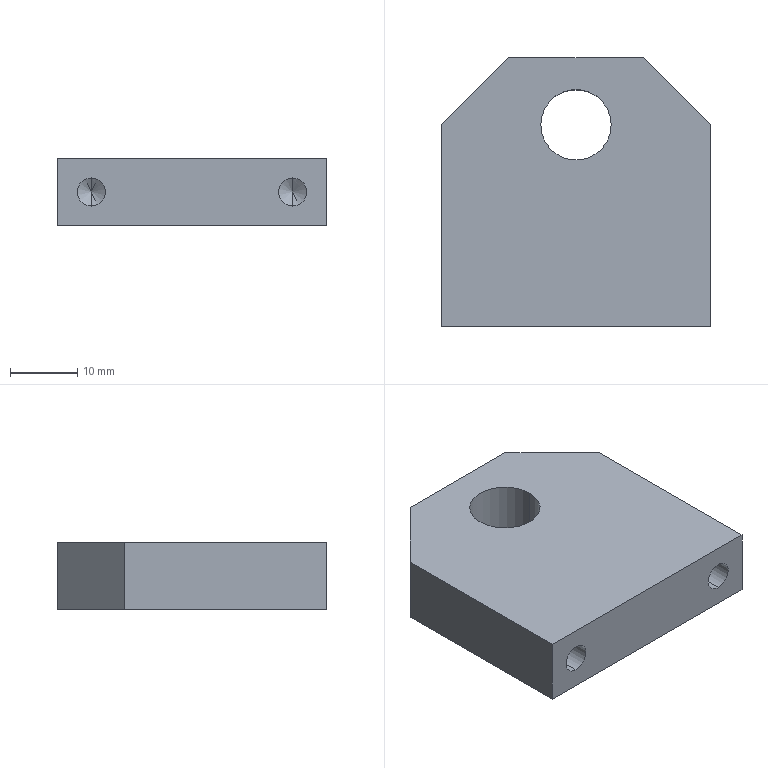Part | SolidWorks | features BaseBody 1 | 1 solid | 18 faces | box 40 x 40 x 10 mm | volume 13735 mm3 | plane 8 | cylinder 6 | cone 4 | commonest cylinder face diameters 4.2 x4 10.5 x2
STEP:
#1=CARTESIAN_POINT('',(-15.,-6.,7.1));
#2=VERTEX_POINT('',#1);
#3=CARTESIAN_POINT('',(-15.,-6.,2.9));
#4=VERTEX_POINT('',#3);
#5=CARTESIAN_POINT('',(-15.,-6.,5.));
#6=DIRECTION('',(0.,-1.,0.));
#7=DIRECTION('',(0.,0.,-1.));
#8=AXIS2_PLACEMENT_3D('',#5,#6,#7);
#9=CIRCLE('',#8,2.1);
#10=EDGE_CURVE('',#2,#4,#9,.T.);
#11=ORIENTED_EDGE('',*,*,#10,.F.);
#12=CARTESIAN_POINT('',(-15.,-20.,7.1));
#13=VERTEX_POINT('',#12);
#14=CARTESIAN_POINT('',(-15.,-20.,7.1));
#15=DIRECTION('',(0.,-1.,0.));
#16=VECTOR('',#15,1000.);
#17=LINE('',#14,#16);
#18=EDGE_CURVE('',#2,#13,#17,.T.);
#19=ORIENTED_EDGE('',*,*,#18,.T.);
#20=CARTESIAN_POINT('',(-15.,-20.,2.9));
#21=VERTEX_POINT('',#20);
#22=CARTESIAN_POINT('',(-15.,-20.,5.));
#23=DIRECTION('',(0.,-1.,0.));
#24=DIRECTION('',(0.,0.,-1.));
#25=AXIS2_PLACEMENT_3D('',#22,#23,#24);
#26=CIRCLE('',#25,2.1);
#27=EDGE_CURVE('',#13,#21,#26,.T.);
#28=ORIENTED_EDGE('',*,*,#27,.T.);
#29=CARTESIAN_POINT('',(-15.,-20.,2.9));
#30=DIRECTION('',(0.,-1.,0.));
#31=VECTOR('',#30,1000.);
#32=LINE('',#29,#31);
#33=EDGE_CURVE('',#4,#21,#32,.T.);
#34=ORIENTED_EDGE('',*,*,#33,.F.);
#35=EDGE_LOOP('',(#11,#19,#28,#34));
#36=FACE_OUTER_BOUND('',#35,.T.);
#37=CARTESIAN_POINT('',(-15.,-20.,5.));
#38=DIRECTION('',(0.,-1.,0.));
#39=DIRECTION('',(0.,0.,-1.));
#40=AXIS2_PLACEMENT_3D('',#37,#38,#39);
#41=CYLINDRICAL_SURFACE('',#40,2.1);
#42=ADVANCED_FACE('',(#36),#41,.F.);
#43=CARTESIAN_POINT('',(-15.,-4.738,5.));
#44=VERTEX_POINT('',#43);
#45=CARTESIAN_POINT('',(-15.,-6.,2.9));
#46=DIRECTION('',(0.,-0.515,-0.8572));
#47=VECTOR('',#46,1000.);
#48=LINE('',#45,#47);
#49=EDGE_CURVE('',#44,#4,#48,.T.);
#50=ORIENTED_EDGE('',*,*,#49,.F.);
#51=CARTESIAN_POINT('',(-15.,-6.,7.1));
#52=DIRECTION('',(0.,-0.515,0.8572));
#53=VECTOR('',#52,1000.);
#54=LINE('',#51,#53);
#55=EDGE_CURVE('',#44,#2,#54,.T.);
#56=ORIENTED_EDGE('',*,*,#55,.T.);
#57=ORIENTED_EDGE('',*,*,#10,.T.);
#58=EDGE_LOOP('',(#50,#56,#57));
#59=FACE_OUTER_BOUND('',#58,.T.);
#60=CARTESIAN_POINT('',(-15.,-6.,5.));
#61=DIRECTION('',(0.,-1.,0.));
#62=DIRECTION('',(0.,0.,-1.));
#63=AXIS2_PLACEMENT_3D('',#60,#61,#62);
#64=CONICAL_SURFACE('',#63,2.1,1.03);
#65=ADVANCED_FACE('',(#59),#64,.F.);
#66=CARTESIAN_POINT('',(15.,-6.,7.1));
#67=VERTEX_POINT('',#66);
#68=CARTESIAN_POINT('',(15.,-6.,2.9));
#69=VERTEX_POINT('',#68);
#70=CARTESIAN_POINT('',(15.,-6.,5.));
#71=DIRECTION('',(0.,-1.,0.));
#72=DIRECTION('',(0.,0.,-1.));
#73=AXIS2_PLACEMENT_3D('',#70,#71,#72);
#74=CIRCLE('',#73,2.1);
#75=EDGE_CURVE('',#67,#69,#74,.T.);
#76=ORIENTED_EDGE('',*,*,#75,.F.);
#77=CARTESIAN_POINT('',(15.,-20.,7.1));
#78=VERTEX_POINT('',#77);
#79=CARTESIAN_POINT('',(15.,-20.,7.1));
#80=DIRECTION('',(0.,-1.,0.));
#81=VECTOR('',#80,1000.);
#82=LINE('',#79,#81);
#83=EDGE_CURVE('',#67,#78,#82,.T.);
#84=ORIENTED_EDGE('',*,*,#83,.T.);
#85=CARTESIAN_POINT('',(15.,-20.,2.9));
#86=VERTEX_POINT('',#85);
#87=CARTESIAN_POINT('',(15.,-20.,5.));
#88=DIRECTION('',(0.,-1.,0.));
#89=DIRECTION('',(0.,0.,-1.));
#90=AXIS2_PLACEMENT_3D('',#87,#88,#89);
#91=CIRCLE('',#90,2.1);
#92=EDGE_CURVE('',#78,#86,#91,.T.);
#93=ORIENTED_EDGE('',*,*,#92,.T.);
#94=CARTESIAN_POINT('',(15.,-20.,2.9));
#95=DIRECTION('',(0.,-1.,0.));
#96=VECTOR('',#95,1000.);
#97=LINE('',#94,#96);
#98=EDGE_CURVE('',#69,#86,#97,.T.);
#99=ORIENTED_EDGE('',*,*,#98,.F.);
#100=EDGE_LOOP('',(#76,#84,#93,#99));
#101=FACE_OUTER_BOUND('',#100,.T.);
#102=CARTESIAN_POINT('',(15.,-20.,5.));
#103=DIRECTION('',(0.,-1.,0.));
#104=DIRECTION('',(0.,0.,-1.));
#105=AXIS2_PLACEMENT_3D('',#102,#103,#104);
#106=CYLINDRICAL_SURFACE('',#105,2.1);
#107=ADVANCED_FACE('',(#101),#106,.F.);
#108=CARTESIAN_POINT('',(15.,-4.738,5.));
#109=VERTEX_POINT('',#108);
#110=CARTESIAN_POINT('',(15.,-6.,2.9));
#111=DIRECTION('',(0.,-0.515,-0.8572));
#112=VECTOR('',#111,1000.);
#113=LINE('',#110,#112);
#114=EDGE_CURVE('',#109,#69,#113,.T.);
#115=ORIENTED_EDGE('',*,*,#114,.F.);
#116=CARTESIAN_POINT('',(15.,-6.,7.1));
#117=DIRECTION('',(0.,-0.515,0.8572));
#118=VECTOR('',#117,1000.);
#119=LINE('',#116,#118);
#120=EDGE_CURVE('',#109,#67,#119,.T.);
#121=ORIENTED_EDGE('',*,*,#120,.T.);
#122=ORIENTED_EDGE('',*,*,#75,.T.);
#123=EDGE_LOOP('',(#115,#121,#122));
#124=FACE_OUTER_BOUND('',#123,.T.);
#125=CARTESIAN_POINT('',(15.,-6.,5.));
#126=DIRECTION('',(0.,-1.,0.));
#127=DIRECTION('',(0.,0.,-1.));
#128=AXIS2_PLACEMENT_3D('',#125,#126,#127);
#129=CONICAL_SURFACE('',#128,2.1,1.03);
#130=ADVANCED_FACE('',(#124),#129,.F.);
#131=CARTESIAN_POINT('',(-5.25,10.,0.));
#132=VERTEX_POINT('',#131);
#133=CARTESIAN_POINT('',(5.25,10.,0.));
#134=VERTEX_POINT('',#133);
#135=CARTESIAN_POINT('',(0.,10.,0.));
#136=DIRECTION('',(0.,0.,1.));
#137=DIRECTION('',(1.,0.,0.));
#138=AXIS2_PLACEMENT_3D('',#135,#136,#137);
#139=CIRCLE('',#138,5.25);
#140=EDGE_CURVE('',#132,#134,#139,.T.);
#141=ORIENTED_EDGE('',*,*,#140,.F.);
#142=CARTESIAN_POINT('',(-5.25,10.,10.));
#143=VERTEX_POINT('',#142);
#144=CARTESIAN_POINT('',(-5.25,10.,0.));
#145=DIRECTION('',(0.,0.,1.));
#146=VECTOR('',#145,1000.);
#147=LINE('',#144,#146);
#148=EDGE_CURVE('',#132,#143,#147,.T.);
#149=ORIENTED_EDGE('',*,*,#148,.T.);
#150=CARTESIAN_POINT('',(5.25,10.,10.));
#151=VERTEX_POINT('',#150);
#152=CARTESIAN_POINT('',(0.,10.,10.));
#153=DIRECTION('',(0.,0.,1.));
#154=DIRECTION('',(1.,0.,0.));
#155=AXIS2_PLACEMENT_3D('',#152,#153,#154);
#156=CIRCLE('',#155,5.25);
#157=EDGE_CURVE('',#143,#151,#156,.T.);
#158=ORIENTED_EDGE('',*,*,#157,.T.);
#159=CARTESIAN_POINT('',(5.25,10.,0.));
#160=DIRECTION('',(0.,0.,1.));
#161=VECTOR('',#160,1000.);
#162=LINE('',#159,#161);
#163=EDGE_CURVE('',#134,#151,#162,.T.);
#164=ORIENTED_EDGE('',*,*,#163,.F.);
#165=EDGE_LOOP('',(#141,#149,#158,#164));
#166=FACE_OUTER_BOUND('',#165,.T.);
#167=CARTESIAN_POINT('',(0.,10.,0.));
#168=DIRECTION('',(0.,0.,1.));
#169=DIRECTION('',(1.,0.,0.));
#170=AXIS2_PLACEMENT_3D('',#167,#168,#169);
#171=CYLINDRICAL_SURFACE('',#170,5.25);
#172=ADVANCED_FACE('',(#166),#171,.F.);
#173=CARTESIAN_POINT('',(-20.,10.,10.));
#174=VERTEX_POINT('',#173);
#175=CARTESIAN_POINT('',(-20.,-20.,10.));
#176=VERTEX_POINT('',#175);
#177=CARTESIAN_POINT('',(-20.,-20.,10.));
#178=DIRECTION('',(0.,-1.,0.));
#179=VECTOR('',#178,1000.);
#180=LINE('',#177,#179);
#181=EDGE_CURVE('',#174,#176,#180,.T.);
#182=ORIENTED_EDGE('',*,*,#181,.F.);
#183=CARTESIAN_POINT('',(-20.,10.,0.));
#184=VERTEX_POINT('',#183);
#185=CARTESIAN_POINT('',(-20.,10.,10.));
#186=DIRECTION('',(0.,0.,-1.));
#187=VECTOR('',#186,1000.);
#188=LINE('',#185,#187);
#189=EDGE_CURVE('',#174,#184,#188,.T.);
#190=ORIENTED_EDGE('',*,*,#189,.T.);
#191=CARTESIAN_POINT('',(-20.,-20.,0.));
#192=VERTEX_POINT('',#191);
#193=CARTESIAN_POINT('',(-20.,-20.,0.));
#194=DIRECTION('',(0.,-1.,0.));
#195=VECTOR('',#194,1000.);
#196=LINE('',#193,#195);
#197=EDGE_CURVE('',#184,#192,#196,.T.);
#198=ORIENTED_EDGE('',*,*,#197,.T.);
#199=CARTESIAN_POINT('',(-20.,-20.,10.));
#200=DIRECTION('',(0.,0.,-1.));
#201=VECTOR('',#200,1000.);
#202=LINE('',#199,#201);
#203=EDGE_CURVE('',#176,#192,#202,.T.);
#204=ORIENTED_EDGE('',*,*,#203,.F.);
#205=EDGE_LOOP('',(#182,#190,#198,#204));
#206=FACE_OUTER_BOUND('',#205,.T.);
#207=CARTESIAN_POINT('',(-20.,-20.,10.));
#208=DIRECTION('',(1.,0.,0.));
#209=DIRECTION('',(0.,0.,-1.));
#210=AXIS2_PLACEMENT_3D('',#207,#208,#209);
#211=PLANE('',#210);
#212=ADVANCED_FACE('',(#206),#211,.F.);
#213=CARTESIAN_POINT('',(-15.,-20.,5.));
#214=DIRECTION('',(0.,-1.,0.));
#215=DIRECTION('',(0.,0.,-1.));
#216=AXIS2_PLACEMENT_3D('',#213,#214,#215);
#217=CIRCLE('',#216,2.1);
#218=EDGE_CURVE('',#21,#13,#217,.T.);
#219=ORIENTED_EDGE('',*,*,#218,.F.);
#220=ORIENTED_EDGE('',*,*,#27,.F.);
#221=EDGE_LOOP('',(#219,#220));
#222=FACE_BOUND('',#221,.T.);
#223=CARTESIAN_POINT('',(15.,-20.,5.));
#224=DIRECTION('',(0.,-1.,0.));
#225=DIRECTION('',(0.,0.,-1.));
#226=AXIS2_PLACEMENT_3D('',#223,#224,#225);
#227=CIRCLE('',#226,2.1);
#228=EDGE_CURVE('',#86,#78,#227,.T.);
#229=ORIENTED_EDGE('',*,*,#228,.F.);
#230=ORIENTED_EDGE('',*,*,#92,.F.);
#231=EDGE_LOOP('',(#229,#230));
#232=FACE_BOUND('',#231,.T.);
#233=CARTESIAN_POINT('',(20.,-20.,0.));
#234=VERTEX_POINT('',#233);
#235=CARTESIAN_POINT('',(20.,-20.,0.));
#236=DIRECTION('',(1.,0.,0.));
#237=VECTOR('',#236,1000.);
#238=LINE('',#235,#237);
#239=EDGE_CURVE('',#192,#234,#238,.T.);
#240=ORIENTED_EDGE('',*,*,#239,.T.);
#241=CARTESIAN_POINT('',(20.,-20.,10.));
#242=VERTEX_POINT('',#241);
#243=CARTESIAN_POINT('',(20.,-20.,10.));
#244=DIRECTION('',(0.,0.,-1.));
#245=VECTOR('',#244,1000.);
#246=LINE('',#243,#245);
#247=EDGE_CURVE('',#242,#234,#246,.T.);
#248=ORIENTED_EDGE('',*,*,#247,.F.);
#249=CARTESIAN_POINT('',(20.,-20.,10.));
#250=DIRECTION('',(1.,0.,0.));
#251=VECTOR('',#250,1000.);
#252=LINE('',#249,#251);
#253=EDGE_CURVE('',#176,#242,#252,.T.);
#254=ORIENTED_EDGE('',*,*,#253,.F.);
#255=ORIENTED_EDGE('',*,*,#203,.T.);
#256=EDGE_LOOP('',(#240,#248,#254,#255));
#257=FACE_OUTER_BOUND('',#256,.T.);
#258=CARTESIAN_POINT('',(20.,-20.,10.));
#259=DIRECTION('',(0.,1.,0.));
#260=DIRECTION('',(-1.,0.,0.));
#261=AXIS2_PLACEMENT_3D('',#258,#259,#260);
#262=PLANE('',#261);
#263=ADVANCED_FACE('',(#222,#232,#257),#262,.F.);
#264=CARTESIAN_POINT('',(20.,10.,0.));
#265=VERTEX_POINT('',#264);
#266=CARTESIAN_POINT('',(20.,-20.,0.));
#267=DIRECTION('',(0.,1.,0.));
#268=VECTOR('',#267,1000.);
#269=LINE('',#266,#268);
#270=EDGE_CURVE('',#234,#265,#269,.T.);
#271=ORIENTED_EDGE('',*,*,#270,.T.);
#272=CARTESIAN_POINT('',(20.,10.,10.));
#273=VERTEX_POINT('',#272);
#274=CARTESIAN_POINT('',(20.,10.,10.));
#275=DIRECTION('',(0.,0.,1.));
#276=VECTOR('',#275,1000.);
#277=LINE('',#274,#276);
#278=EDGE_CURVE('',#265,#273,#277,.T.);
#279=ORIENTED_EDGE('',*,*,#278,.T.);
#280=CARTESIAN_POINT('',(20.,-20.,10.));
#281=DIRECTION('',(0.,1.,0.));
#282=VECTOR('',#281,1000.);
#283=LINE('',#280,#282);
#284=EDGE_CURVE('',#242,#273,#283,.T.);
#285=ORIENTED_EDGE('',*,*,#284,.F.);
#286=ORIENTED_EDGE('',*,*,#247,.T.);
#287=EDGE_LOOP('',(#271,#279,#285,#286));
#288=FACE_OUTER_BOUND('',#287,.T.);
#289=CARTESIAN_POINT('',(20.,-20.,10.));
#290=DIRECTION('',(-1.,0.,0.));
#291=DIRECTION('',(0.,0.,1.));
#292=AXIS2_PLACEMENT_3D('',#289,#290,#291);
#293=PLANE('',#292);
#294=ADVANCED_FACE('',(#288),#293,.F.);
#295=CARTESIAN_POINT('',(10.,20.,10.));
#296=VERTEX_POINT('',#295);
#297=CARTESIAN_POINT('',(-10.,20.,10.));
#298=VERTEX_POINT('',#297);
#299=CARTESIAN_POINT('',(20.,20.,10.));
#300=DIRECTION('',(-1.,0.,0.));
#301=VECTOR('',#300,1000.);
#302=LINE('',#299,#301);
#303=EDGE_CURVE('',#296,#298,#302,.T.);
#304=ORIENTED_EDGE('',*,*,#303,.F.);
#305=CARTESIAN_POINT('',(10.,20.,0.));
#306=VERTEX_POINT('',#305);
#307=CARTESIAN_POINT('',(10.,20.,10.));
#308=DIRECTION('',(0.,0.,-1.));
#309=VECTOR('',#308,1000.);
#310=LINE('',#307,#309);
#311=EDGE_CURVE('',#296,#306,#310,.T.);
#312=ORIENTED_EDGE('',*,*,#311,.T.);
#313=CARTESIAN_POINT('',(-10.,20.,0.));
#314=VERTEX_POINT('',#313);
#315=CARTESIAN_POINT('',(20.,20.,0.));
#316=DIRECTION('',(-1.,0.,0.));
#317=VECTOR('',#316,1000.);
#318=LINE('',#315,#317);
#319=EDGE_CURVE('',#306,#314,#318,.T.);
#320=ORIENTED_EDGE('',*,*,#319,.T.);
#321=CARTESIAN_POINT('',(-10.,20.,10.));
#322=DIRECTION('',(0.,0.,1.));
#323=VECTOR('',#322,1000.);
#324=LINE('',#321,#323);
#325=EDGE_CURVE('',#314,#298,#324,.T.);
#326=ORIENTED_EDGE('',*,*,#325,.T.);
#327=EDGE_LOOP('',(#304,#312,#320,#326));
#328=FACE_OUTER_BOUND('',#327,.T.);
#329=CARTESIAN_POINT('',(20.,20.,10.));
#330=DIRECTION('',(0.,-1.,0.));
#331=DIRECTION('',(1.,0.,0.));
#332=AXIS2_PLACEMENT_3D('',#329,#330,#331);
#333=PLANE('',#332);
#334=ADVANCED_FACE('',(#328),#333,.F.);
#335=CARTESIAN_POINT('',(0.,10.,10.));
#336=DIRECTION('',(0.,0.,1.));
#337=DIRECTION('',(1.,0.,0.));
#338=AXIS2_PLACEMENT_3D('',#335,#336,#337);
#339=CIRCLE('',#338,5.25);
#340=EDGE_CURVE('',#151,#143,#339,.T.);
#341=ORIENTED_EDGE('',*,*,#340,.F.);
#342=ORIENTED_EDGE('',*,*,#157,.F.);
#343=EDGE_LOOP('',(#341,#342));
#344=FACE_BOUND('',#343,.T.);
#345=ORIENTED_EDGE('',*,*,#284,.T.);
#346=CARTESIAN_POINT('',(15.,15.,10.));
#347=DIRECTION('',(-0.7071,0.7071,0.));
#348=VECTOR('',#347,1000.);
#349=LINE('',#346,#348);
#350=EDGE_CURVE('',#273,#296,#349,.T.);
#351=ORIENTED_EDGE('',*,*,#350,.T.);
#352=ORIENTED_EDGE('',*,*,#303,.T.);
#353=CARTESIAN_POINT('',(-15.,15.,10.));
#354=DIRECTION('',(-0.7071,-0.7071,0.));
#355=VECTOR('',#354,1000.);
#356=LINE('',#353,#355);
#357=EDGE_CURVE('',#298,#174,#356,.T.);
#358=ORIENTED_EDGE('',*,*,#357,.T.);
#359=ORIENTED_EDGE('',*,*,#181,.T.);
#360=ORIENTED_EDGE('',*,*,#253,.T.);
#361=EDGE_LOOP('',(#345,#351,#352,#358,#359,#360));
#362=FACE_OUTER_BOUND('',#361,.T.);
#363=CARTESIAN_POINT('',(0.,0.,10.));
#364=DIRECTION('',(0.,0.,1.));
#365=DIRECTION('',(1.,0.,0.));
#366=AXIS2_PLACEMENT_3D('',#363,#364,#365);
#367=PLANE('',#366);
#368=ADVANCED_FACE('',(#344,#362),#367,.T.);
#369=CARTESIAN_POINT('',(0.,10.,0.));
#370=DIRECTION('',(0.,0.,1.));
#371=DIRECTION('',(1.,0.,0.));
#372=AXIS2_PLACEMENT_3D('',#369,#370,#371);
#373=CIRCLE('',#372,5.25);
#374=EDGE_CURVE('',#134,#132,#373,.T.);
#375=ORIENTED_EDGE('',*,*,#374,.T.);
#376=ORIENTED_EDGE('',*,*,#140,.T.);
#377=EDGE_LOOP('',(#375,#376));
#378=FACE_BOUND('',#377,.T.);
#379=ORIENTED_EDGE('',*,*,#319,.F.);
#380=CARTESIAN_POINT('',(10.,20.,0.));
#381=DIRECTION('',(0.7071,-0.7071,0.));
#382=VECTOR('',#381,1000.);
#383=LINE('',#380,#382);
#384=EDGE_CURVE('',#306,#265,#383,.T.);
#385=ORIENTED_EDGE('',*,*,#384,.T.);
#386=ORIENTED_EDGE('',*,*,#270,.F.);
#387=ORIENTED_EDGE('',*,*,#239,.F.);
#388=ORIENTED_EDGE('',*,*,#197,.F.);
#389=CARTESIAN_POINT('',(-20.,10.,0.));
#390=DIRECTION('',(0.7071,0.7071,0.));
#391=VECTOR('',#390,1000.);
#392=LINE('',#389,#391);
#393=EDGE_CURVE('',#184,#314,#392,.T.);
#394=ORIENTED_EDGE('',*,*,#393,.T.);
#395=EDGE_LOOP('',(#379,#385,#386,#387,#388,#394));
#396=FACE_OUTER_BOUND('',#395,.T.);
#397=CARTESIAN_POINT('',(0.,0.,0.));
#398=DIRECTION('',(0.,0.,1.));
#399=DIRECTION('',(1.,0.,0.));
#400=AXIS2_PLACEMENT_3D('',#397,#398,#399);
#401=PLANE('',#400);
#402=ADVANCED_FACE('',(#378,#396),#401,.F.);
#403=ORIENTED_EDGE('',*,*,#148,.F.);
#404=ORIENTED_EDGE('',*,*,#374,.F.);
#405=ORIENTED_EDGE('',*,*,#163,.T.);
#406=ORIENTED_EDGE('',*,*,#340,.T.);
#407=EDGE_LOOP('',(#403,#404,#405,#406));
#408=FACE_OUTER_BOUND('',#407,.T.);
#409=CARTESIAN_POINT('',(0.,10.,0.));
#410=DIRECTION('',(0.,0.,1.));
#411=DIRECTION('',(1.,0.,0.));
#412=AXIS2_PLACEMENT_3D('',#409,#410,#411);
#413=CYLINDRICAL_SURFACE('',#412,5.25);
#414=ADVANCED_FACE('',(#408),#413,.F.);
#415=ORIENTED_EDGE('',*,*,#350,.F.);
#416=ORIENTED_EDGE('',*,*,#278,.F.);
#417=ORIENTED_EDGE('',*,*,#384,.F.);
#418=ORIENTED_EDGE('',*,*,#311,.F.);
#419=EDGE_LOOP('',(#415,#416,#417,#418));
#420=FACE_OUTER_BOUND('',#419,.T.);
#421=CARTESIAN_POINT('',(10.,20.,10.));
#422=DIRECTION('',(-0.7071,-0.7071,0.));
#423=DIRECTION('',(0.,0.,-1.));
#424=AXIS2_PLACEMENT_3D('',#421,#422,#423);
#425=PLANE('',#424);
#426=ADVANCED_FACE('',(#420),#425,.F.);
#427=ORIENTED_EDGE('',*,*,#357,.F.);
#428=ORIENTED_EDGE('',*,*,#325,.F.);
#429=ORIENTED_EDGE('',*,*,#393,.F.);
#430=ORIENTED_EDGE('',*,*,#189,.F.);
#431=EDGE_LOOP('',(#427,#428,#429,#430));
#432=FACE_OUTER_BOUND('',#431,.T.);
#433=CARTESIAN_POINT('',(-20.,10.,10.));
#434=DIRECTION('',(0.7071,-0.7071,0.));
#435=DIRECTION('',(0.,0.,-1.));
#436=AXIS2_PLACEMENT_3D('',#433,#434,#435);
#437=PLANE('',#436);
#438=ADVANCED_FACE('',(#432),#437,.F.);
#439=ORIENTED_EDGE('',*,*,#120,.F.);
#440=ORIENTED_EDGE('',*,*,#114,.T.);
#441=CARTESIAN_POINT('',(15.,-6.,5.));
#442=DIRECTION('',(0.,-1.,0.));
#443=DIRECTION('',(0.,0.,-1.));
#444=AXIS2_PLACEMENT_3D('',#441,#442,#443);
#445=CIRCLE('',#444,2.1);
#446=EDGE_CURVE('',#69,#67,#445,.T.);
#447=ORIENTED_EDGE('',*,*,#446,.T.);
#448=EDGE_LOOP('',(#439,#440,#447));
#449=FACE_OUTER_BOUND('',#448,.T.);
#450=CARTESIAN_POINT('',(15.,-6.,5.));
#451=DIRECTION('',(0.,-1.,0.));
#452=DIRECTION('',(0.,0.,-1.));
#453=AXIS2_PLACEMENT_3D('',#450,#451,#452);
#454=CONICAL_SURFACE('',#453,2.1,1.03);
#455=ADVANCED_FACE('',(#449),#454,.F.);
#456=ORIENTED_EDGE('',*,*,#83,.F.);
#457=ORIENTED_EDGE('',*,*,#446,.F.);
#458=ORIENTED_EDGE('',*,*,#98,.T.);
#459=ORIENTED_EDGE('',*,*,#228,.T.);
#460=EDGE_LOOP('',(#456,#457,#458,#459));
#461=FACE_OUTER_BOUND('',#460,.T.);
#462=CARTESIAN_POINT('',(15.,-20.,5.));
#463=DIRECTION('',(0.,-1.,0.));
#464=DIRECTION('',(0.,0.,-1.));
#465=AXIS2_PLACEMENT_3D('',#462,#463,#464);
#466=CYLINDRICAL_SURFACE('',#465,2.1);
#467=ADVANCED_FACE('',(#461),#466,.F.);
#468=ORIENTED_EDGE('',*,*,#55,.F.);
#469=ORIENTED_EDGE('',*,*,#49,.T.);
#470=CARTESIAN_POINT('',(-15.,-6.,5.));
#471=DIRECTION('',(0.,-1.,0.));
#472=DIRECTION('',(0.,0.,-1.));
#473=AXIS2_PLACEMENT_3D('',#470,#471,#472);
#474=CIRCLE('',#473,2.1);
#475=EDGE_CURVE('',#4,#2,#474,.T.);
#476=ORIENTED_EDGE('',*,*,#475,.T.);
#477=EDGE_LOOP('',(#468,#469,#476));
#478=FACE_OUTER_BOUND('',#477,.T.);
#479=CARTESIAN_POINT('',(-15.,-6.,5.));
#480=DIRECTION('',(0.,-1.,0.));
#481=DIRECTION('',(0.,0.,-1.));
#482=AXIS2_PLACEMENT_3D('',#479,#480,#481);
#483=CONICAL_SURFACE('',#482,2.1,1.03);
#484=ADVANCED_FACE('',(#478),#483,.F.);
#485=ORIENTED_EDGE('',*,*,#18,.F.);
#486=ORIENTED_EDGE('',*,*,#475,.F.);
#487=ORIENTED_EDGE('',*,*,#33,.T.);
#488=ORIENTED_EDGE('',*,*,#218,.T.);
#489=EDGE_LOOP('',(#485,#486,#487,#488));
#490=FACE_OUTER_BOUND('',#489,.T.);
#491=CARTESIAN_POINT('',(-15.,-20.,5.));
#492=DIRECTION('',(0.,-1.,0.));
#493=DIRECTION('',(0.,0.,-1.));
#494=AXIS2_PLACEMENT_3D('',#491,#492,#493);
#495=CYLINDRICAL_SURFACE('',#494,2.1);
#496=ADVANCED_FACE('',(#490),#495,.F.);
#497=CLOSED_SHELL('',(#42,#65,#107,#130,#172,#212,#263,#294,#334,#368,#402,#414,#426,#438,#455,#467,#484,#496));
#498=MANIFOLD_SOLID_BREP('',#497);
#499=CARTESIAN_POINT('',(0.,0.,0.));
#500=DIRECTION('',(0.,0.,1.));
#501=DIRECTION('',(1.,0.,0.));
#502=AXIS2_PLACEMENT_3D('',#499,#500,#501);
#503=(LENGTH_UNIT()NAMED_UNIT(*)SI_UNIT(.MILLI.,.METRE.));
#504=UNCERTAINTY_MEASURE_WITH_UNIT(LENGTH_MEASURE(0.00001),#503,'','');
#505=(NAMED_UNIT(*)PLANE_ANGLE_UNIT()SI_UNIT($,.RADIAN.));
#506=(NAMED_UNIT(*)SI_UNIT($,.STERADIAN.)SOLID_ANGLE_UNIT());
#507=(GEOMETRIC_REPRESENTATION_CONTEXT(3)GLOBAL_UNCERTAINTY_ASSIGNED_CONTEXT((#504))GLOBAL_UNIT_ASSIGNED_CONTEXT((#503,#505,#506))REPRESENTATION_CONTEXT('',''));
#508=ADVANCED_BREP_SHAPE_REPRESENTATION('',(#498,#502),#507);